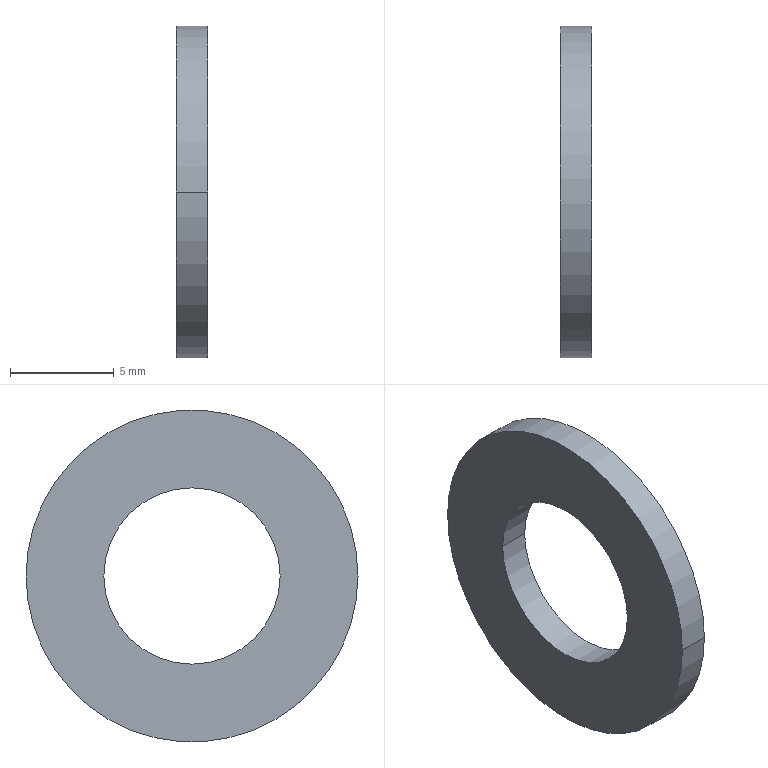Part | STEP file | [Anti-tilt]-Part-1 | 1 solid | 6 faces | box 1.5 x 16 x 16 mm | volume 216.475 mm3 | cylinder 4 | plane 2 | commonest cylinder face diameters 8.5 x2 16 x2
STEP:
#1=CARTESIAN_POINT('',(53.91,-6.25,11.));
#2=VERTEX_POINT('',#1);
#3=CARTESIAN_POINT('',(53.91,-14.75,11.));
#4=VERTEX_POINT('',#3);
#5=CARTESIAN_POINT('',(53.91,-10.5,11.));
#6=DIRECTION('',(-1.,0.,0.));
#7=DIRECTION('',(0.,-1.,0.));
#8=AXIS2_PLACEMENT_3D('',#5,#6,#7);
#9=CIRCLE('',#8,4.25);
#10=EDGE_CURVE('',#2,#4,#9,.T.);
#11=ORIENTED_EDGE('',*,*,#10,.F.);
#12=CARTESIAN_POINT('',(52.41,-6.25,11.));
#13=VERTEX_POINT('',#12);
#14=CARTESIAN_POINT('',(53.91,-6.25,11.));
#15=DIRECTION('',(-1.,0.,0.));
#16=VECTOR('',#15,1000.);
#17=LINE('',#14,#16);
#18=EDGE_CURVE('',#2,#13,#17,.T.);
#19=ORIENTED_EDGE('',*,*,#18,.T.);
#20=CARTESIAN_POINT('',(52.41,-14.75,11.));
#21=VERTEX_POINT('',#20);
#22=CARTESIAN_POINT('',(52.41,-10.5,11.));
#23=DIRECTION('',(1.,0.,0.));
#24=DIRECTION('',(0.,1.,0.));
#25=AXIS2_PLACEMENT_3D('',#22,#23,#24);
#26=CIRCLE('',#25,4.25);
#27=EDGE_CURVE('',#21,#13,#26,.T.);
#28=ORIENTED_EDGE('',*,*,#27,.F.);
#29=CARTESIAN_POINT('',(53.91,-14.75,11.));
#30=DIRECTION('',(-1.,0.,0.));
#31=VECTOR('',#30,1000.);
#32=LINE('',#29,#31);
#33=EDGE_CURVE('',#4,#21,#32,.T.);
#34=ORIENTED_EDGE('',*,*,#33,.F.);
#35=EDGE_LOOP('',(#11,#19,#28,#34));
#36=FACE_OUTER_BOUND('',#35,.T.);
#37=CARTESIAN_POINT('',(53.91,-10.5,11.));
#38=DIRECTION('',(-1.,0.,0.));
#39=DIRECTION('',(0.,-1.,0.));
#40=AXIS2_PLACEMENT_3D('',#37,#38,#39);
#41=CYLINDRICAL_SURFACE('',#40,4.25);
#42=ADVANCED_FACE('',(#36),#41,.F.);
#43=CARTESIAN_POINT('',(53.91,-18.5,11.));
#44=VERTEX_POINT('',#43);
#45=CARTESIAN_POINT('',(53.91,-2.5,11.));
#46=VERTEX_POINT('',#45);
#47=CARTESIAN_POINT('',(53.91,-10.5,11.));
#48=DIRECTION('',(-1.,0.,0.));
#49=DIRECTION('',(0.,-1.,0.));
#50=AXIS2_PLACEMENT_3D('',#47,#48,#49);
#51=CIRCLE('',#50,8.);
#52=EDGE_CURVE('',#44,#46,#51,.T.);
#53=ORIENTED_EDGE('',*,*,#52,.T.);
#54=CARTESIAN_POINT('',(52.41,-2.5,11.));
#55=VERTEX_POINT('',#54);
#56=CARTESIAN_POINT('',(53.91,-2.5,11.));
#57=DIRECTION('',(-1.,0.,0.));
#58=VECTOR('',#57,1000.);
#59=LINE('',#56,#58);
#60=EDGE_CURVE('',#46,#55,#59,.T.);
#61=ORIENTED_EDGE('',*,*,#60,.T.);
#62=CARTESIAN_POINT('',(52.41,-18.5,11.));
#63=VERTEX_POINT('',#62);
#64=CARTESIAN_POINT('',(52.41,-10.5,11.));
#65=DIRECTION('',(1.,0.,0.));
#66=DIRECTION('',(0.,1.,0.));
#67=AXIS2_PLACEMENT_3D('',#64,#65,#66);
#68=CIRCLE('',#67,8.);
#69=EDGE_CURVE('',#55,#63,#68,.T.);
#70=ORIENTED_EDGE('',*,*,#69,.T.);
#71=CARTESIAN_POINT('',(53.91,-18.5,11.));
#72=DIRECTION('',(-1.,0.,0.));
#73=VECTOR('',#72,1000.);
#74=LINE('',#71,#73);
#75=EDGE_CURVE('',#44,#63,#74,.T.);
#76=ORIENTED_EDGE('',*,*,#75,.F.);
#77=EDGE_LOOP('',(#53,#61,#70,#76));
#78=FACE_OUTER_BOUND('',#77,.T.);
#79=CARTESIAN_POINT('',(53.91,-10.5,11.));
#80=DIRECTION('',(-1.,0.,0.));
#81=DIRECTION('',(0.,-1.,0.));
#82=AXIS2_PLACEMENT_3D('',#79,#80,#81);
#83=CYLINDRICAL_SURFACE('',#82,8.);
#84=ADVANCED_FACE('',(#78),#83,.T.);
#85=ORIENTED_EDGE('',*,*,#27,.T.);
#86=CARTESIAN_POINT('',(52.41,-10.5,11.));
#87=DIRECTION('',(1.,0.,0.));
#88=DIRECTION('',(0.,1.,0.));
#89=AXIS2_PLACEMENT_3D('',#86,#87,#88);
#90=CIRCLE('',#89,4.25);
#91=EDGE_CURVE('',#13,#21,#90,.T.);
#92=ORIENTED_EDGE('',*,*,#91,.T.);
#93=EDGE_LOOP('',(#85,#92));
#94=FACE_BOUND('',#93,.T.);
#95=CARTESIAN_POINT('',(52.41,-10.5,11.));
#96=DIRECTION('',(1.,0.,0.));
#97=DIRECTION('',(0.,1.,0.));
#98=AXIS2_PLACEMENT_3D('',#95,#96,#97);
#99=CIRCLE('',#98,8.);
#100=EDGE_CURVE('',#63,#55,#99,.T.);
#101=ORIENTED_EDGE('',*,*,#100,.F.);
#102=ORIENTED_EDGE('',*,*,#69,.F.);
#103=EDGE_LOOP('',(#101,#102));
#104=FACE_OUTER_BOUND('',#103,.T.);
#105=CARTESIAN_POINT('',(52.41,-10.5,11.));
#106=DIRECTION('',(-1.,0.,0.));
#107=DIRECTION('',(0.,-1.,0.));
#108=AXIS2_PLACEMENT_3D('',#105,#106,#107);
#109=PLANE('',#108);
#110=ADVANCED_FACE('',(#94,#104),#109,.T.);
#111=CARTESIAN_POINT('',(53.91,-10.5,11.));
#112=DIRECTION('',(-1.,0.,0.));
#113=DIRECTION('',(0.,-1.,0.));
#114=AXIS2_PLACEMENT_3D('',#111,#112,#113);
#115=CIRCLE('',#114,4.25);
#116=EDGE_CURVE('',#4,#2,#115,.T.);
#117=ORIENTED_EDGE('',*,*,#116,.T.);
#118=ORIENTED_EDGE('',*,*,#10,.T.);
#119=EDGE_LOOP('',(#117,#118));
#120=FACE_BOUND('',#119,.T.);
#121=ORIENTED_EDGE('',*,*,#52,.F.);
#122=CARTESIAN_POINT('',(53.91,-10.5,11.));
#123=DIRECTION('',(-1.,0.,0.));
#124=DIRECTION('',(0.,-1.,0.));
#125=AXIS2_PLACEMENT_3D('',#122,#123,#124);
#126=CIRCLE('',#125,8.);
#127=EDGE_CURVE('',#46,#44,#126,.T.);
#128=ORIENTED_EDGE('',*,*,#127,.F.);
#129=EDGE_LOOP('',(#121,#128));
#130=FACE_OUTER_BOUND('',#129,.T.);
#131=CARTESIAN_POINT('',(53.91,-10.5,11.));
#132=DIRECTION('',(1.,0.,0.));
#133=DIRECTION('',(0.,1.,0.));
#134=AXIS2_PLACEMENT_3D('',#131,#132,#133);
#135=PLANE('',#134);
#136=ADVANCED_FACE('',(#120,#130),#135,.T.);
#137=ORIENTED_EDGE('',*,*,#60,.F.);
#138=ORIENTED_EDGE('',*,*,#127,.T.);
#139=ORIENTED_EDGE('',*,*,#75,.T.);
#140=ORIENTED_EDGE('',*,*,#100,.T.);
#141=EDGE_LOOP('',(#137,#138,#139,#140));
#142=FACE_OUTER_BOUND('',#141,.T.);
#143=CARTESIAN_POINT('',(53.91,-10.5,11.));
#144=DIRECTION('',(-1.,0.,0.));
#145=DIRECTION('',(0.,-1.,0.));
#146=AXIS2_PLACEMENT_3D('',#143,#144,#145);
#147=CYLINDRICAL_SURFACE('',#146,8.);
#148=ADVANCED_FACE('',(#142),#147,.T.);
#149=ORIENTED_EDGE('',*,*,#18,.F.);
#150=ORIENTED_EDGE('',*,*,#116,.F.);
#151=ORIENTED_EDGE('',*,*,#33,.T.);
#152=ORIENTED_EDGE('',*,*,#91,.F.);
#153=EDGE_LOOP('',(#149,#150,#151,#152));
#154=FACE_OUTER_BOUND('',#153,.T.);
#155=CARTESIAN_POINT('',(53.91,-10.5,11.));
#156=DIRECTION('',(-1.,0.,0.));
#157=DIRECTION('',(0.,-1.,0.));
#158=AXIS2_PLACEMENT_3D('',#155,#156,#157);
#159=CYLINDRICAL_SURFACE('',#158,4.25);
#160=ADVANCED_FACE('',(#154),#159,.F.);
#161=CLOSED_SHELL('',(#42,#84,#110,#136,#148,#160));
#162=MANIFOLD_SOLID_BREP('',#161);
#163=CARTESIAN_POINT('',(0.,0.,0.));
#164=DIRECTION('',(0.,0.,1.));
#165=DIRECTION('',(1.,0.,0.));
#166=AXIS2_PLACEMENT_3D('',#163,#164,#165);
#167=(LENGTH_UNIT()NAMED_UNIT(*)SI_UNIT(.MILLI.,.METRE.));
#168=UNCERTAINTY_MEASURE_WITH_UNIT(LENGTH_MEASURE(0.00001),#167,'','');
#169=(NAMED_UNIT(*)PLANE_ANGLE_UNIT()SI_UNIT($,.RADIAN.));
#170=(NAMED_UNIT(*)SI_UNIT($,.STERADIAN.)SOLID_ANGLE_UNIT());
#171=(GEOMETRIC_REPRESENTATION_CONTEXT(3)GLOBAL_UNCERTAINTY_ASSIGNED_CONTEXT((#168))GLOBAL_UNIT_ASSIGNED_CONTEXT((#167,#169,#170))REPRESENTATION_CONTEXT('',''));
#172=ADVANCED_BREP_SHAPE_REPRESENTATION('',(#162,#166),#171);